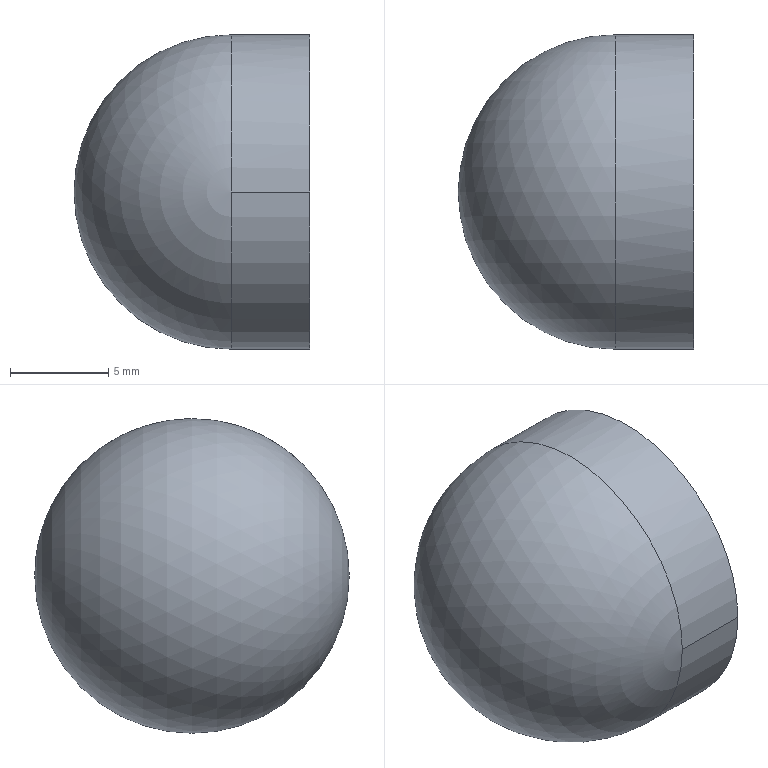Part | STEP file | Positioning_id1610_x_t | 1 solid | 4 faces | box 12 x 16 x 16 mm | volume 1877 mm3 | cylinder 2 | sphere 1 | plane 1 | commonest cylinder face diameters 16 x2
STEP:
#1=CARTESIAN_POINT('',(0.,0.,0.));
#2=DIRECTION('',(0.,0.,1.));
#3=DIRECTION('',(1.,0.,0.));
#4=AXIS2_PLACEMENT_3D('',#1,#2,#3);
#5=CARTESIAN_POINT('',(-781.002,-209.5,139.532));
#6=VERTEX_POINT('',#5);
#7=CARTESIAN_POINT('',(-781.002,-201.5,131.532));
#8=VERTEX_POINT('',#7);
#9=CARTESIAN_POINT('',(-781.002,-201.5,139.532));
#10=DIRECTION('',(1.,0.,0.));
#11=DIRECTION('',(0.,-1.,0.));
#12=AXIS2_PLACEMENT_3D('',#9,#10,#11);
#13=CIRCLE('',#12,8.);
#14=CARTESIAN_POINT('',(-781.002,-201.5,139.532));
#15=DIRECTION('',(0.,1.,0.));
#16=DIRECTION('',(-1.,0.,0.));
#17=AXIS2_PLACEMENT_3D('',#14,#15,#16);
#18=SPHERICAL_SURFACE('',#17,8.);
#19=CARTESIAN_POINT('',(4.712,-1.571));
#20=CARTESIAN_POINT('',(4.712,-1.547));
#21=CARTESIAN_POINT('',(4.712,-1.499));
#22=CARTESIAN_POINT('',(4.712,-1.428));
#23=CARTESIAN_POINT('',(4.712,-1.357));
#24=CARTESIAN_POINT('',(4.712,-1.285));
#25=CARTESIAN_POINT('',(4.712,-1.214));
#26=CARTESIAN_POINT('',(4.712,-1.142));
#27=CARTESIAN_POINT('',(4.712,-1.071));
#28=CARTESIAN_POINT('',(4.712,-0.9996));
#29=CARTESIAN_POINT('',(4.712,-0.9282));
#30=CARTESIAN_POINT('',(4.712,-0.8568));
#31=CARTESIAN_POINT('',(4.712,-0.7854));
#32=CARTESIAN_POINT('',(4.712,-0.714));
#33=CARTESIAN_POINT('',(4.712,-0.6426));
#34=CARTESIAN_POINT('',(4.712,-0.5712));
#35=CARTESIAN_POINT('',(4.712,-0.4998));
#36=CARTESIAN_POINT('',(4.712,-0.4284));
#37=CARTESIAN_POINT('',(4.712,-0.357));
#38=CARTESIAN_POINT('',(4.712,-0.2856));
#39=CARTESIAN_POINT('',(4.712,-0.2142));
#40=CARTESIAN_POINT('',(4.712,-0.1428));
#41=CARTESIAN_POINT('',(4.712,-0.0714));
#42=CARTESIAN_POINT('',(4.712,-0.0238));
#43=CARTESIAN_POINT('',(4.712,0.));
#44=B_SPLINE_CURVE_WITH_KNOTS('',3,(#19,#20,#21,#22,#23,#24,#25,#26,#27,#28,#29,#30,#31,#32,#33,#34,#35,#36,#37,#38,#39,#40,#41,#42,#43),.UNSPECIFIED.,.F.,.F.,(4,1,1,1,1,1,1,1,1,1,1,1,1,1,1,1,1,1,1,1,1,1,4),(0.,0.0714,0.1428,0.2142,0.2856,0.357,0.4284,0.4998,0.5712,0.6426,0.714,0.7854,0.8568,0.9282,0.9996,1.071,1.142,1.214,1.285,1.357,1.428,1.499,1.571),.QUASI_UNIFORM_KNOTS.);
#45=(GEOMETRIC_REPRESENTATION_CONTEXT(2)PARAMETRIC_REPRESENTATION_CONTEXT()REPRESENTATION_CONTEXT('',''));
#46=DEFINITIONAL_REPRESENTATION('',(#44),#45);
#47=PCURVE('',#18,#46);
#48=CARTESIAN_POINT('',(-774.002,-201.5,139.532));
#49=DIRECTION('',(1.,0.,0.));
#50=DIRECTION('',(0.,1.,0.));
#51=AXIS2_PLACEMENT_3D('',#48,#49,#50);
#52=CYLINDRICAL_SURFACE('',#51,8.);
#53=CARTESIAN_POINT('',(3.142,-7.));
#54=DIRECTION('',(1.,0.));
#55=VECTOR('',#54,1.);
#56=LINE('',#53,#55);
#57=(GEOMETRIC_REPRESENTATION_CONTEXT(2)PARAMETRIC_REPRESENTATION_CONTEXT()REPRESENTATION_CONTEXT('',''));
#58=DEFINITIONAL_REPRESENTATION('',(#56),#57);
#59=PCURVE('',#52,#58);
#60=SURFACE_CURVE('',#13,(#47,#59),.PCURVE_S1.);
#61=EDGE_CURVE('',#6,#8,#60,.T.);
#62=ORIENTED_EDGE('',*,*,#61,.F.);
#63=CARTESIAN_POINT('',(-781.002,-201.5,147.532));
#64=VERTEX_POINT('',#63);
#65=CARTESIAN_POINT('',(-781.002,-201.5,139.532));
#66=DIRECTION('',(1.,0.,0.));
#67=DIRECTION('',(0.,0.,1.));
#68=AXIS2_PLACEMENT_3D('',#65,#66,#67);
#69=CIRCLE('',#68,8.);
#70=CARTESIAN_POINT('',(7.854,0.));
#71=CARTESIAN_POINT('',(7.854,-0.0238));
#72=CARTESIAN_POINT('',(7.854,-0.0714));
#73=CARTESIAN_POINT('',(7.854,-0.1428));
#74=CARTESIAN_POINT('',(7.854,-0.2142));
#75=CARTESIAN_POINT('',(7.854,-0.2856));
#76=CARTESIAN_POINT('',(7.854,-0.357));
#77=CARTESIAN_POINT('',(7.854,-0.4284));
#78=CARTESIAN_POINT('',(7.854,-0.4998));
#79=CARTESIAN_POINT('',(7.854,-0.5712));
#80=CARTESIAN_POINT('',(7.854,-0.6426));
#81=CARTESIAN_POINT('',(7.854,-0.714));
#82=CARTESIAN_POINT('',(7.854,-0.7854));
#83=CARTESIAN_POINT('',(7.854,-0.8568));
#84=CARTESIAN_POINT('',(7.854,-0.9282));
#85=CARTESIAN_POINT('',(7.854,-0.9996));
#86=CARTESIAN_POINT('',(7.854,-1.071));
#87=CARTESIAN_POINT('',(7.854,-1.142));
#88=CARTESIAN_POINT('',(7.854,-1.214));
#89=CARTESIAN_POINT('',(7.854,-1.285));
#90=CARTESIAN_POINT('',(7.854,-1.357));
#91=CARTESIAN_POINT('',(7.854,-1.428));
#92=CARTESIAN_POINT('',(7.854,-1.499));
#93=CARTESIAN_POINT('',(7.854,-1.547));
#94=CARTESIAN_POINT('',(7.854,-1.571));
#95=B_SPLINE_CURVE_WITH_KNOTS('',3,(#70,#71,#72,#73,#74,#75,#76,#77,#78,#79,#80,#81,#82,#83,#84,#85,#86,#87,#88,#89,#90,#91,#92,#93,#94),.UNSPECIFIED.,.F.,.F.,(4,1,1,1,1,1,1,1,1,1,1,1,1,1,1,1,1,1,1,1,1,1,4),(0.,0.0714,0.1428,0.2142,0.2856,0.357,0.4284,0.4998,0.5712,0.6426,0.714,0.7854,0.8568,0.9282,0.9996,1.071,1.142,1.214,1.285,1.357,1.428,1.499,1.571),.QUASI_UNIFORM_KNOTS.);
#96=(GEOMETRIC_REPRESENTATION_CONTEXT(2)PARAMETRIC_REPRESENTATION_CONTEXT()REPRESENTATION_CONTEXT('',''));
#97=DEFINITIONAL_REPRESENTATION('',(#95),#96);
#98=PCURVE('',#18,#97);
#99=CARTESIAN_POINT('',(-774.002,-201.5,139.532));
#100=DIRECTION('',(1.,0.,0.));
#101=DIRECTION('',(0.,1.,0.));
#102=AXIS2_PLACEMENT_3D('',#99,#100,#101);
#103=CYLINDRICAL_SURFACE('',#102,8.);
#104=CARTESIAN_POINT('',(1.571,-7.));
#105=DIRECTION('',(1.,0.));
#106=VECTOR('',#105,1.);
#107=LINE('',#104,#106);
#108=(GEOMETRIC_REPRESENTATION_CONTEXT(2)PARAMETRIC_REPRESENTATION_CONTEXT()REPRESENTATION_CONTEXT('',''));
#109=DEFINITIONAL_REPRESENTATION('',(#107),#108);
#110=PCURVE('',#103,#109);
#111=SURFACE_CURVE('',#69,(#98,#110),.PCURVE_S1.);
#112=EDGE_CURVE('',#64,#6,#111,.T.);
#113=ORIENTED_EDGE('',*,*,#112,.F.);
#114=CARTESIAN_POINT('',(-781.002,-193.5,139.532));
#115=VERTEX_POINT('',#114);
#116=CARTESIAN_POINT('',(-781.002,-201.5,139.532));
#117=DIRECTION('',(1.,0.,0.));
#118=DIRECTION('',(0.,1.,0.));
#119=AXIS2_PLACEMENT_3D('',#116,#117,#118);
#120=CIRCLE('',#119,8.);
#121=CARTESIAN_POINT('',(7.854,1.571));
#122=CARTESIAN_POINT('',(7.854,1.547));
#123=CARTESIAN_POINT('',(7.854,1.499));
#124=CARTESIAN_POINT('',(7.854,1.428));
#125=CARTESIAN_POINT('',(7.854,1.357));
#126=CARTESIAN_POINT('',(7.854,1.285));
#127=CARTESIAN_POINT('',(7.854,1.214));
#128=CARTESIAN_POINT('',(7.854,1.142));
#129=CARTESIAN_POINT('',(7.854,1.071));
#130=CARTESIAN_POINT('',(7.854,0.9996));
#131=CARTESIAN_POINT('',(7.854,0.9282));
#132=CARTESIAN_POINT('',(7.854,0.8568));
#133=CARTESIAN_POINT('',(7.854,0.7854));
#134=CARTESIAN_POINT('',(7.854,0.714));
#135=CARTESIAN_POINT('',(7.854,0.6426));
#136=CARTESIAN_POINT('',(7.854,0.5712));
#137=CARTESIAN_POINT('',(7.854,0.4998));
#138=CARTESIAN_POINT('',(7.854,0.4284));
#139=CARTESIAN_POINT('',(7.854,0.357));
#140=CARTESIAN_POINT('',(7.854,0.2856));
#141=CARTESIAN_POINT('',(7.854,0.2142));
#142=CARTESIAN_POINT('',(7.854,0.1428));
#143=CARTESIAN_POINT('',(7.854,0.0714));
#144=CARTESIAN_POINT('',(7.854,0.0238));
#145=CARTESIAN_POINT('',(7.854,0.));
#146=B_SPLINE_CURVE_WITH_KNOTS('',3,(#121,#122,#123,#124,#125,#126,#127,#128,#129,#130,#131,#132,#133,#134,#135,#136,#137,#138,#139,#140,#141,#142,#143,#144,#145),.UNSPECIFIED.,.F.,.F.,(4,1,1,1,1,1,1,1,1,1,1,1,1,1,1,1,1,1,1,1,1,1,4),(0.,0.0714,0.1428,0.2142,0.2856,0.357,0.4284,0.4998,0.5712,0.6426,0.714,0.7854,0.8568,0.9282,0.9996,1.071,1.142,1.214,1.285,1.357,1.428,1.499,1.571),.QUASI_UNIFORM_KNOTS.);
#147=(GEOMETRIC_REPRESENTATION_CONTEXT(2)PARAMETRIC_REPRESENTATION_CONTEXT()REPRESENTATION_CONTEXT('',''));
#148=DEFINITIONAL_REPRESENTATION('',(#146),#147);
#149=PCURVE('',#18,#148);
#150=CARTESIAN_POINT('',(0.,-7.));
#151=DIRECTION('',(1.,0.));
#152=VECTOR('',#151,1.);
#153=LINE('',#150,#152);
#154=(GEOMETRIC_REPRESENTATION_CONTEXT(2)PARAMETRIC_REPRESENTATION_CONTEXT()REPRESENTATION_CONTEXT('',''));
#155=DEFINITIONAL_REPRESENTATION('',(#153),#154);
#156=PCURVE('',#103,#155);
#157=SURFACE_CURVE('',#120,(#149,#156),.PCURVE_S1.);
#158=EDGE_CURVE('',#115,#64,#157,.T.);
#159=ORIENTED_EDGE('',*,*,#158,.F.);
#160=CARTESIAN_POINT('',(-781.002,-201.5,139.532));
#161=DIRECTION('',(1.,0.,0.));
#162=DIRECTION('',(0.,0.,-1.));
#163=AXIS2_PLACEMENT_3D('',#160,#161,#162);
#164=CIRCLE('',#163,8.);
#165=CARTESIAN_POINT('',(4.712,0.));
#166=CARTESIAN_POINT('',(4.712,0.0238));
#167=CARTESIAN_POINT('',(4.712,0.0714));
#168=CARTESIAN_POINT('',(4.712,0.1428));
#169=CARTESIAN_POINT('',(4.712,0.2142));
#170=CARTESIAN_POINT('',(4.712,0.2856));
#171=CARTESIAN_POINT('',(4.712,0.357));
#172=CARTESIAN_POINT('',(4.712,0.4284));
#173=CARTESIAN_POINT('',(4.712,0.4998));
#174=CARTESIAN_POINT('',(4.712,0.5712));
#175=CARTESIAN_POINT('',(4.712,0.6426));
#176=CARTESIAN_POINT('',(4.712,0.714));
#177=CARTESIAN_POINT('',(4.712,0.7854));
#178=CARTESIAN_POINT('',(4.712,0.8568));
#179=CARTESIAN_POINT('',(4.712,0.9282));
#180=CARTESIAN_POINT('',(4.712,0.9996));
#181=CARTESIAN_POINT('',(4.712,1.071));
#182=CARTESIAN_POINT('',(4.712,1.142));
#183=CARTESIAN_POINT('',(4.712,1.214));
#184=CARTESIAN_POINT('',(4.712,1.285));
#185=CARTESIAN_POINT('',(4.712,1.357));
#186=CARTESIAN_POINT('',(4.712,1.428));
#187=CARTESIAN_POINT('',(4.712,1.499));
#188=CARTESIAN_POINT('',(4.712,1.547));
#189=CARTESIAN_POINT('',(4.712,1.571));
#190=B_SPLINE_CURVE_WITH_KNOTS('',3,(#165,#166,#167,#168,#169,#170,#171,#172,#173,#174,#175,#176,#177,#178,#179,#180,#181,#182,#183,#184,#185,#186,#187,#188,#189),.UNSPECIFIED.,.F.,.F.,(4,1,1,1,1,1,1,1,1,1,1,1,1,1,1,1,1,1,1,1,1,1,4),(0.,0.0714,0.1428,0.2142,0.2856,0.357,0.4284,0.4998,0.5712,0.6426,0.714,0.7854,0.8568,0.9282,0.9996,1.071,1.142,1.214,1.285,1.357,1.428,1.499,1.571),.QUASI_UNIFORM_KNOTS.);
#191=(GEOMETRIC_REPRESENTATION_CONTEXT(2)PARAMETRIC_REPRESENTATION_CONTEXT()REPRESENTATION_CONTEXT('',''));
#192=DEFINITIONAL_REPRESENTATION('',(#190),#191);
#193=PCURVE('',#18,#192);
#194=CARTESIAN_POINT('',(4.712,-7.));
#195=DIRECTION('',(1.,0.));
#196=VECTOR('',#195,1.);
#197=LINE('',#194,#196);
#198=(GEOMETRIC_REPRESENTATION_CONTEXT(2)PARAMETRIC_REPRESENTATION_CONTEXT()REPRESENTATION_CONTEXT('',''));
#199=DEFINITIONAL_REPRESENTATION('',(#197),#198);
#200=PCURVE('',#52,#199);
#201=SURFACE_CURVE('',#164,(#193,#200),.PCURVE_S1.);
#202=EDGE_CURVE('',#8,#115,#201,.T.);
#203=ORIENTED_EDGE('',*,*,#202,.F.);
#204=EDGE_LOOP('',(#62,#113,#159,#203));
#205=FACE_BOUND('',#204,.T.);
#206=ADVANCED_FACE('',(#205),#18,.T.);
#207=CARTESIAN_POINT('',(-777.002,-193.5,139.532));
#208=VERTEX_POINT('',#207);
#209=CARTESIAN_POINT('',(-777.002,-193.5,139.532));
#210=DIRECTION('',(1.,0.,0.));
#211=VECTOR('',#210,1.);
#212=LINE('',#209,#211);
#213=CARTESIAN_POINT('',(6.283,-3.));
#214=DIRECTION('',(0.,1.));
#215=VECTOR('',#214,1.);
#216=LINE('',#213,#215);
#217=(GEOMETRIC_REPRESENTATION_CONTEXT(2)PARAMETRIC_REPRESENTATION_CONTEXT()REPRESENTATION_CONTEXT('',''));
#218=DEFINITIONAL_REPRESENTATION('',(#216),#217);
#219=PCURVE('',#52,#218);
#220=CARTESIAN_POINT('',(0.,-3.));
#221=DIRECTION('',(0.,1.));
#222=VECTOR('',#221,1.);
#223=LINE('',#220,#222);
#224=(GEOMETRIC_REPRESENTATION_CONTEXT(2)PARAMETRIC_REPRESENTATION_CONTEXT()REPRESENTATION_CONTEXT('',''));
#225=DEFINITIONAL_REPRESENTATION('',(#223),#224);
#226=PCURVE('',#103,#225);
#227=SURFACE_CURVE('',#212,(#219,#226),.PCURVE_S1.);
#228=EDGE_CURVE('',#115,#208,#227,.T.);
#229=ORIENTED_EDGE('',*,*,#228,.T.);
#230=CARTESIAN_POINT('',(-777.002,-209.5,139.532));
#231=VERTEX_POINT('',#230);
#232=CARTESIAN_POINT('',(-777.002,-201.5,139.532));
#233=DIRECTION('',(-1.,0.,0.));
#234=DIRECTION('',(0.,1.,0.));
#235=AXIS2_PLACEMENT_3D('',#232,#233,#234);
#236=CIRCLE('',#235,8.);
#237=CARTESIAN_POINT('',(6.283,-3.));
#238=DIRECTION('',(-1.,0.));
#239=VECTOR('',#238,1.);
#240=LINE('',#237,#239);
#241=(GEOMETRIC_REPRESENTATION_CONTEXT(2)PARAMETRIC_REPRESENTATION_CONTEXT()REPRESENTATION_CONTEXT('',''));
#242=DEFINITIONAL_REPRESENTATION('',(#240),#241);
#243=PCURVE('',#52,#242);
#244=CARTESIAN_POINT('',(-777.002,-201.5,139.532));
#245=DIRECTION('',(1.,0.,0.));
#246=DIRECTION('',(0.,-1.,0.));
#247=AXIS2_PLACEMENT_3D('',#244,#245,#246);
#248=PLANE('',#247);
#249=CARTESIAN_POINT('',(-8.,0.));
#250=CARTESIAN_POINT('',(-8.,13.856));
#251=CARTESIAN_POINT('',(4.,6.928));
#252=CARTESIAN_POINT('',(16.,0.));
#253=CARTESIAN_POINT('',(4.,-6.928));
#254=CARTESIAN_POINT('',(-8.,-13.856));
#255=CARTESIAN_POINT('',(-8.,0.));
#256=(BOUNDED_CURVE()B_SPLINE_CURVE(2,(#249,#250,#251,#252,#253,#254,#255),.UNSPECIFIED.,.T.,.F.)B_SPLINE_CURVE_WITH_KNOTS((1,2,2,2,2,1),(-2.094,0.,2.094,4.189,6.283,8.378),.UNSPECIFIED.)CURVE()GEOMETRIC_REPRESENTATION_ITEM()RATIONAL_B_SPLINE_CURVE((1.,0.5,1.,0.5,1.,0.5,1.))REPRESENTATION_ITEM(''));
#257=(GEOMETRIC_REPRESENTATION_CONTEXT(2)PARAMETRIC_REPRESENTATION_CONTEXT()REPRESENTATION_CONTEXT('',''));
#258=DEFINITIONAL_REPRESENTATION('',(#256),#257);
#259=PCURVE('',#248,#258);
#260=SURFACE_CURVE('',#236,(#243,#259),.PCURVE_S1.);
#261=EDGE_CURVE('',#208,#231,#260,.T.);
#262=ORIENTED_EDGE('',*,*,#261,.T.);
#263=CARTESIAN_POINT('',(-777.002,-209.5,139.532));
#264=DIRECTION('',(-1.,0.,0.));
#265=VECTOR('',#264,1.);
#266=LINE('',#263,#265);
#267=CARTESIAN_POINT('',(3.142,-3.));
#268=DIRECTION('',(0.,-1.));
#269=VECTOR('',#268,1.);
#270=LINE('',#267,#269);
#271=(GEOMETRIC_REPRESENTATION_CONTEXT(2)PARAMETRIC_REPRESENTATION_CONTEXT()REPRESENTATION_CONTEXT('',''));
#272=DEFINITIONAL_REPRESENTATION('',(#270),#271);
#273=PCURVE('',#52,#272);
#274=CARTESIAN_POINT('',(3.142,-3.));
#275=DIRECTION('',(0.,-1.));
#276=VECTOR('',#275,1.);
#277=LINE('',#274,#276);
#278=(GEOMETRIC_REPRESENTATION_CONTEXT(2)PARAMETRIC_REPRESENTATION_CONTEXT()REPRESENTATION_CONTEXT('',''));
#279=DEFINITIONAL_REPRESENTATION('',(#277),#278);
#280=PCURVE('',#103,#279);
#281=SURFACE_CURVE('',#266,(#273,#280),.PCURVE_S1.);
#282=EDGE_CURVE('',#231,#6,#281,.T.);
#283=ORIENTED_EDGE('',*,*,#282,.T.);
#284=ORIENTED_EDGE('',*,*,#61,.T.);
#285=ORIENTED_EDGE('',*,*,#202,.T.);
#286=EDGE_LOOP('',(#229,#262,#283,#284,#285));
#287=FACE_BOUND('',#286,.T.);
#288=ADVANCED_FACE('',(#287),#52,.T.);
#289=CARTESIAN_POINT('',(-777.002,-209.5,139.532));
#290=CARTESIAN_POINT('',(-777.002,-209.5,147.532));
#291=CARTESIAN_POINT('',(-777.002,-201.5,151.532));
#292=CARTESIAN_POINT('',(-777.002,-193.5,147.532));
#293=CARTESIAN_POINT('',(-777.002,-193.5,139.532));
#294=(BOUNDED_CURVE()B_SPLINE_CURVE(4,(#289,#290,#291,#292,#293),.UNSPECIFIED.,.F.,.F.)B_SPLINE_CURVE_WITH_KNOTS((5,5),(0.,1.),.PIECEWISE_BEZIER_KNOTS.)CURVE()GEOMETRIC_REPRESENTATION_ITEM()RATIONAL_B_SPLINE_CURVE((1.,0.7071,0.6667,0.7071,1.))REPRESENTATION_ITEM(''));
#295=CARTESIAN_POINT('',(8.,0.));
#296=CARTESIAN_POINT('',(8.,-8.));
#297=CARTESIAN_POINT('',(0.,-12.));
#298=CARTESIAN_POINT('',(-8.,-8.));
#299=CARTESIAN_POINT('',(-8.,0.));
#300=(BOUNDED_CURVE()B_SPLINE_CURVE(4,(#295,#296,#297,#298,#299),.UNSPECIFIED.,.F.,.F.)B_SPLINE_CURVE_WITH_KNOTS((5,5),(0.,1.),.PIECEWISE_BEZIER_KNOTS.)CURVE()GEOMETRIC_REPRESENTATION_ITEM()RATIONAL_B_SPLINE_CURVE((1.,0.7071,0.6667,0.7071,1.))REPRESENTATION_ITEM(''));
#301=(GEOMETRIC_REPRESENTATION_CONTEXT(2)PARAMETRIC_REPRESENTATION_CONTEXT()REPRESENTATION_CONTEXT('',''));
#302=DEFINITIONAL_REPRESENTATION('',(#300),#301);
#303=PCURVE('',#248,#302);
#304=CARTESIAN_POINT('',(3.142,-3.));
#305=CARTESIAN_POINT('',(3.099,-3.));
#306=CARTESIAN_POINT('',(3.012,-3.));
#307=CARTESIAN_POINT('',(2.878,-3.));
#308=CARTESIAN_POINT('',(2.742,-3.));
#309=CARTESIAN_POINT('',(2.602,-3.));
#310=CARTESIAN_POINT('',(2.46,-3.));
#311=CARTESIAN_POINT('',(2.316,-3.));
#312=CARTESIAN_POINT('',(2.169,-3.));
#313=CARTESIAN_POINT('',(2.021,-3.));
#314=CARTESIAN_POINT('',(1.872,-3.));
#315=CARTESIAN_POINT('',(1.721,-3.));
#316=CARTESIAN_POINT('',(1.571,-3.));
#317=CARTESIAN_POINT('',(1.42,-3.));
#318=CARTESIAN_POINT('',(1.27,-3.));
#319=CARTESIAN_POINT('',(1.121,-3.));
#320=CARTESIAN_POINT('',(0.9725,-3.));
#321=CARTESIAN_POINT('',(0.8261,-3.));
#322=CARTESIAN_POINT('',(0.6816,-3.));
#323=CARTESIAN_POINT('',(0.5394,-3.));
#324=CARTESIAN_POINT('',(0.3999,-3.));
#325=CARTESIAN_POINT('',(0.2633,-3.));
#326=CARTESIAN_POINT('',(0.1297,-3.));
#327=CARTESIAN_POINT('',(0.04285,-3.));
#328=CARTESIAN_POINT('',(0.,-3.));
#329=B_SPLINE_CURVE_WITH_KNOTS('',3,(#304,#305,#306,#307,#308,#309,#310,#311,#312,#313,#314,#315,#316,#317,#318,#319,#320,#321,#322,#323,#324,#325,#326,#327,#328),.UNSPECIFIED.,.F.,.F.,(4,1,1,1,1,1,1,1,1,1,1,1,1,1,1,1,1,1,1,1,1,1,4),(0.,0.04545,0.09091,0.1364,0.1818,0.2273,0.2727,0.3182,0.3636,0.4091,0.4545,0.5,0.5455,0.5909,0.6364,0.6818,0.7273,0.7727,0.8182,0.8636,0.9091,0.9545,1.),.QUASI_UNIFORM_KNOTS.);
#330=(GEOMETRIC_REPRESENTATION_CONTEXT(2)PARAMETRIC_REPRESENTATION_CONTEXT()REPRESENTATION_CONTEXT('',''));
#331=DEFINITIONAL_REPRESENTATION('',(#329),#330);
#332=PCURVE('',#103,#331);
#333=SURFACE_CURVE('',#294,(#303,#332),.PCURVE_S1.);
#334=EDGE_CURVE('',#231,#208,#333,.T.);
#335=ORIENTED_EDGE('',*,*,#334,.F.);
#336=ORIENTED_EDGE('',*,*,#261,.F.);
#337=EDGE_LOOP('',(#335,#336));
#338=FACE_BOUND('',#337,.T.);
#339=ADVANCED_FACE('',(#338),#248,.T.);
#340=ORIENTED_EDGE('',*,*,#334,.T.);
#341=ORIENTED_EDGE('',*,*,#228,.F.);
#342=ORIENTED_EDGE('',*,*,#158,.T.);
#343=ORIENTED_EDGE('',*,*,#112,.T.);
#344=ORIENTED_EDGE('',*,*,#282,.F.);
#345=EDGE_LOOP('',(#340,#341,#342,#343,#344));
#346=FACE_BOUND('',#345,.T.);
#347=ADVANCED_FACE('',(#346),#103,.T.);
#348=CLOSED_SHELL('',(#206,#288,#339,#347));
#349=MANIFOLD_SOLID_BREP('',#348);
#350=(LENGTH_UNIT()NAMED_UNIT(*)SI_UNIT(.MILLI.,.METRE.));
#351=UNCERTAINTY_MEASURE_WITH_UNIT(LENGTH_MEASURE(0.0000001),#350,'','');
#352=(NAMED_UNIT(*)PLANE_ANGLE_UNIT()SI_UNIT($,.RADIAN.));
#353=(NAMED_UNIT(*)SI_UNIT($,.STERADIAN.)SOLID_ANGLE_UNIT());
#354=(GEOMETRIC_REPRESENTATION_CONTEXT(3)GLOBAL_UNCERTAINTY_ASSIGNED_CONTEXT((#351))GLOBAL_UNIT_ASSIGNED_CONTEXT((#350,#352,#353))REPRESENTATION_CONTEXT('',''));
#355=ADVANCED_BREP_SHAPE_REPRESENTATION('',(#4,#349),#354);